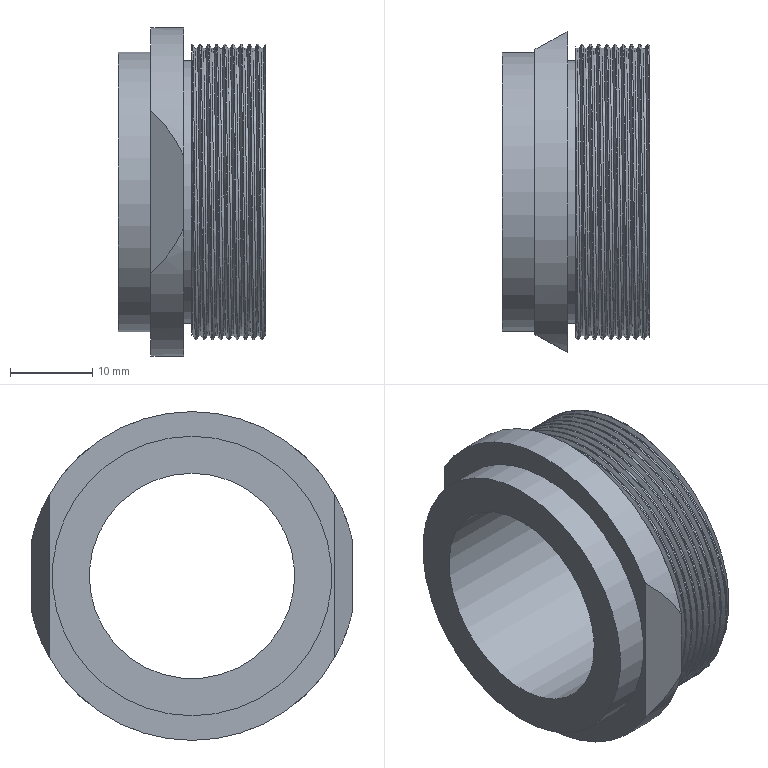Part | NX | features DATUM_CSYS 3, SKETCH 2, THREADS 2, EXTRUDE 1, SWP104 1 | 1 solid | 19 faces | box 18 x 39.042 x 40 mm | volume 9368 mm3 | plane 8 | cylinder 7 | spline 4 | commonest cylinder face diameters 40 x2 25 x1 32 x1 34 x1 35 x1 36 x1